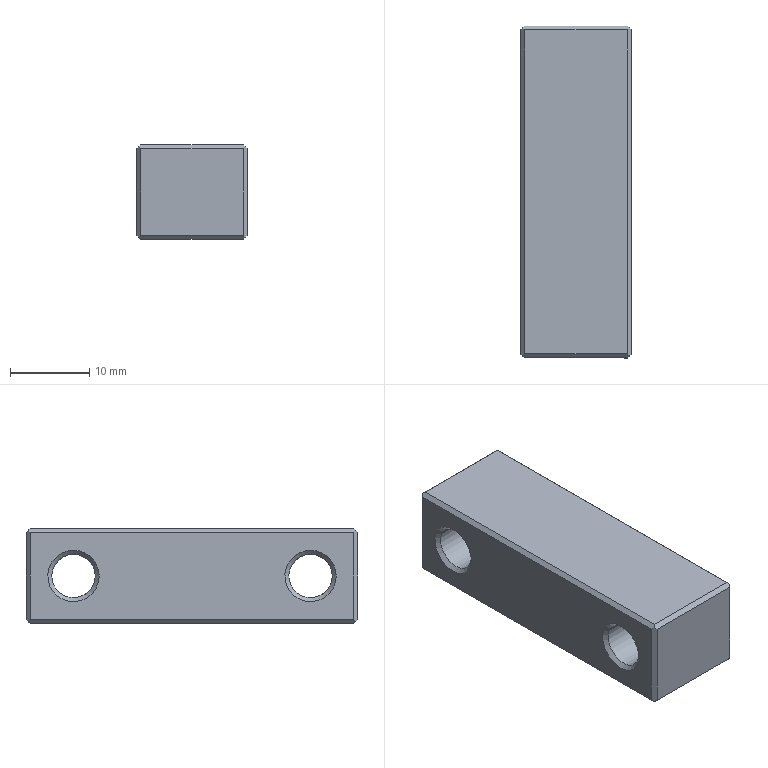Part | NX | 1 solid | 22 faces | box 14 x 42 x 12 mm | volume 6353 mm3 | plane 18 | cone 2 | cylinder 2 | commonest cylinder face diameters 5.5 x2
STEP:
#1=CARTESIAN_POINT('',(-39.202,6.721,154.477));
#2=VERTEX_POINT('',#1);
#3=CARTESIAN_POINT('',(-26.202,6.721,154.477));
#4=VERTEX_POINT('',#3);
#5=CARTESIAN_POINT('',(-1.702,6.721,154.477));
#6=DIRECTION('',(1.,0.,0.));
#7=VECTOR('',#6,1000.);
#8=LINE('',#5,#7);
#9=EDGE_CURVE('',#2,#4,#8,.T.);
#10=ORIENTED_EDGE('',*,*,#9,.T.);
#11=CARTESIAN_POINT('',(-26.202,47.721,154.477));
#12=VERTEX_POINT('',#11);
#13=CARTESIAN_POINT('',(-26.202,48.221,154.477));
#14=DIRECTION('',(0.,1.,0.));
#15=VECTOR('',#14,1000.);
#16=LINE('',#13,#15);
#17=EDGE_CURVE('',#4,#12,#16,.T.);
#18=ORIENTED_EDGE('',*,*,#17,.T.);
#19=CARTESIAN_POINT('',(-39.202,47.721,154.477));
#20=VERTEX_POINT('',#19);
#21=CARTESIAN_POINT('',(-1.702,47.721,154.477));
#22=DIRECTION('',(-1.,0.,0.));
#23=VECTOR('',#22,1000.);
#24=LINE('',#21,#23);
#25=EDGE_CURVE('',#12,#20,#24,.T.);
#26=ORIENTED_EDGE('',*,*,#25,.T.);
#27=CARTESIAN_POINT('',(-39.202,48.221,154.477));
#28=DIRECTION('',(0.,-1.,0.));
#29=VECTOR('',#28,1000.);
#30=LINE('',#27,#29);
#31=EDGE_CURVE('',#20,#2,#30,.T.);
#32=ORIENTED_EDGE('',*,*,#31,.T.);
#33=EDGE_LOOP('',(#10,#18,#26,#32));
#34=FACE_BOUND('',#33,.T.);
#35=CARTESIAN_POINT('',(-33.202,48.221,154.477));
#36=DIRECTION('',(0.,0.,-1.));
#37=DIRECTION('',(0.,-1.,0.));
#38=AXIS2_PLACEMENT_3D('',#35,#36,#37);
#39=PLANE('',#38);
#40=ADVANCED_FACE('',(#34),#39,.F.);
#41=CARTESIAN_POINT('',(-25.952,47.971,154.227));
#42=VERTEX_POINT('',#41);
#43=CARTESIAN_POINT('',(-41.43,32.492,169.705));
#44=DIRECTION('',(0.5774,0.5774,-0.5774));
#45=VECTOR('',#44,1000.);
#46=LINE('',#43,#45);
#47=EDGE_CURVE('',#12,#42,#46,.T.);
#48=ORIENTED_EDGE('',*,*,#47,.T.);
#49=CARTESIAN_POINT('',(-26.202,48.221,153.977));
#50=VERTEX_POINT('',#49);
#51=CARTESIAN_POINT('',(-29.702,51.721,150.477));
#52=DIRECTION('',(-0.5774,0.5774,-0.5774));
#53=VECTOR('',#52,1000.);
#54=LINE('',#51,#53);
#55=EDGE_CURVE('',#42,#50,#54,.T.);
#56=ORIENTED_EDGE('',*,*,#55,.T.);
#57=CARTESIAN_POINT('',(-39.202,48.221,153.977));
#58=VERTEX_POINT('',#57);
#59=CARTESIAN_POINT('',(-22.702,48.221,153.977));
#60=DIRECTION('',(1.,0.,0.));
#61=VECTOR('',#60,1000.);
#62=LINE('',#59,#61);
#63=EDGE_CURVE('',#58,#50,#62,.T.);
#64=ORIENTED_EDGE('',*,*,#63,.F.);
#65=CARTESIAN_POINT('',(-39.452,47.971,154.227));
#66=VERTEX_POINT('',#65);
#67=CARTESIAN_POINT('',(-39.202,48.221,153.977));
#68=DIRECTION('',(-0.5774,-0.5774,0.5774));
#69=VECTOR('',#68,1000.);
#70=LINE('',#67,#69);
#71=EDGE_CURVE('',#58,#66,#70,.T.);
#72=ORIENTED_EDGE('',*,*,#71,.T.);
#73=CARTESIAN_POINT('',(-39.452,47.971,154.227));
#74=DIRECTION('',(0.5774,-0.5774,0.5774));
#75=VECTOR('',#74,1000.);
#76=LINE('',#73,#75);
#77=EDGE_CURVE('',#66,#20,#76,.T.);
#78=ORIENTED_EDGE('',*,*,#77,.T.);
#79=ORIENTED_EDGE('',*,*,#25,.F.);
#80=EDGE_LOOP('',(#48,#56,#64,#72,#78,#79));
#81=FACE_BOUND('',#80,.T.);
#82=CARTESIAN_POINT('',(-1.702,48.221,153.977));
#83=DIRECTION('',(0.,-0.7071,-0.7071));
#84=DIRECTION('',(0.,-0.7071,0.7071));
#85=AXIS2_PLACEMENT_3D('',#82,#83,#84);
#86=PLANE('',#85);
#87=ADVANCED_FACE('',(#81),#86,.F.);
#88=CARTESIAN_POINT('',(-39.202,48.221,142.977));
#89=VERTEX_POINT('',#88);
#90=CARTESIAN_POINT('',(-39.202,48.221,142.477));
#91=DIRECTION('',(0.,0.,1.));
#92=VECTOR('',#91,1000.);
#93=LINE('',#90,#92);
#94=EDGE_CURVE('',#89,#58,#93,.T.);
#95=ORIENTED_EDGE('',*,*,#94,.F.);
#96=CARTESIAN_POINT('',(-39.452,47.971,142.727));
#97=VERTEX_POINT('',#96);
#98=CARTESIAN_POINT('',(-39.452,47.971,142.727));
#99=DIRECTION('',(0.5774,0.5774,0.5774));
#100=VECTOR('',#99,1000.);
#101=LINE('',#98,#100);
#102=EDGE_CURVE('',#97,#89,#101,.T.);
#103=ORIENTED_EDGE('',*,*,#102,.F.);
#104=CARTESIAN_POINT('',(-39.702,47.721,142.977));
#105=VERTEX_POINT('',#104);
#106=CARTESIAN_POINT('',(-39.702,47.721,142.977));
#107=DIRECTION('',(0.5774,0.5774,-0.5774));
#108=VECTOR('',#107,1000.);
#109=LINE('',#106,#108);
#110=EDGE_CURVE('',#105,#97,#109,.T.);
#111=ORIENTED_EDGE('',*,*,#110,.F.);
#112=CARTESIAN_POINT('',(-39.702,47.721,153.977));
#113=VERTEX_POINT('',#112);
#114=CARTESIAN_POINT('',(-39.702,47.721,142.977));
#115=DIRECTION('',(0.,0.,1.));
#116=VECTOR('',#115,1000.);
#117=LINE('',#114,#116);
#118=EDGE_CURVE('',#105,#113,#117,.T.);
#119=ORIENTED_EDGE('',*,*,#118,.T.);
#120=CARTESIAN_POINT('',(-39.702,47.721,153.977));
#121=DIRECTION('',(0.5774,0.5774,0.5774));
#122=VECTOR('',#121,1000.);
#123=LINE('',#120,#122);
#124=EDGE_CURVE('',#113,#66,#123,.T.);
#125=ORIENTED_EDGE('',*,*,#124,.T.);
#126=ORIENTED_EDGE('',*,*,#71,.F.);
#127=EDGE_LOOP('',(#95,#103,#111,#119,#125,#126));
#128=FACE_BOUND('',#127,.T.);
#129=CARTESIAN_POINT('',(-39.202,48.221,163.477));
#130=DIRECTION('',(0.7071,-0.7071,0.));
#131=DIRECTION('',(0.,0.,-1.));
#132=AXIS2_PLACEMENT_3D('',#129,#130,#131);
#133=PLANE('',#132);
#134=ADVANCED_FACE('',(#128),#133,.F.);
#135=ORIENTED_EDGE('',*,*,#31,.F.);
#136=ORIENTED_EDGE('',*,*,#77,.F.);
#137=ORIENTED_EDGE('',*,*,#124,.F.);
#138=CARTESIAN_POINT('',(-39.702,6.721,153.977));
#139=VERTEX_POINT('',#138);
#140=CARTESIAN_POINT('',(-39.702,48.221,153.977));
#141=DIRECTION('',(0.,-1.,0.));
#142=VECTOR('',#141,1000.);
#143=LINE('',#140,#142);
#144=EDGE_CURVE('',#113,#139,#143,.T.);
#145=ORIENTED_EDGE('',*,*,#144,.T.);
#146=CARTESIAN_POINT('',(-39.452,6.471,154.227));
#147=VERTEX_POINT('',#146);
#148=CARTESIAN_POINT('',(-39.702,6.721,153.977));
#149=DIRECTION('',(0.5774,-0.5774,0.5774));
#150=VECTOR('',#149,1000.);
#151=LINE('',#148,#150);
#152=EDGE_CURVE('',#139,#147,#151,.T.);
#153=ORIENTED_EDGE('',*,*,#152,.T.);
#154=CARTESIAN_POINT('',(-39.452,6.471,154.227));
#155=DIRECTION('',(0.5774,0.5774,0.5774));
#156=VECTOR('',#155,1000.);
#157=LINE('',#154,#156);
#158=EDGE_CURVE('',#147,#2,#157,.T.);
#159=ORIENTED_EDGE('',*,*,#158,.T.);
#160=EDGE_LOOP('',(#135,#136,#137,#145,#153,#159));
#161=FACE_BOUND('',#160,.T.);
#162=CARTESIAN_POINT('',(-39.702,48.221,153.977));
#163=DIRECTION('',(0.7071,0.,-0.7071));
#164=DIRECTION('',(0.,-1.,0.));
#165=AXIS2_PLACEMENT_3D('',#162,#163,#164);
#166=PLANE('',#165);
#167=ADVANCED_FACE('',(#161),#166,.F.);
#168=CARTESIAN_POINT('',(-39.202,6.221,142.977));
#169=VERTEX_POINT('',#168);
#170=CARTESIAN_POINT('',(-39.202,6.221,153.977));
#171=VERTEX_POINT('',#170);
#172=CARTESIAN_POINT('',(-39.202,6.221,142.477));
#173=DIRECTION('',(0.,0.,1.));
#174=VECTOR('',#173,1000.);
#175=LINE('',#172,#174);
#176=EDGE_CURVE('',#169,#171,#175,.T.);
#177=ORIENTED_EDGE('',*,*,#176,.T.);
#178=CARTESIAN_POINT('',(-39.202,6.221,153.977));
#179=DIRECTION('',(-0.5774,0.5774,0.5774));
#180=VECTOR('',#179,1000.);
#181=LINE('',#178,#180);
#182=EDGE_CURVE('',#171,#147,#181,.T.);
#183=ORIENTED_EDGE('',*,*,#182,.T.);
#184=ORIENTED_EDGE('',*,*,#152,.F.);
#185=CARTESIAN_POINT('',(-39.702,6.721,142.977));
#186=VERTEX_POINT('',#185);
#187=CARTESIAN_POINT('',(-39.702,6.721,142.977));
#188=DIRECTION('',(0.,0.,-1.));
#189=VECTOR('',#188,1000.);
#190=LINE('',#187,#189);
#191=EDGE_CURVE('',#139,#186,#190,.T.);
#192=ORIENTED_EDGE('',*,*,#191,.T.);
#193=CARTESIAN_POINT('',(-39.452,6.471,142.727));
#194=VERTEX_POINT('',#193);
#195=CARTESIAN_POINT('',(-39.452,6.471,142.727));
#196=DIRECTION('',(-0.5774,0.5774,0.5774));
#197=VECTOR('',#196,1000.);
#198=LINE('',#195,#197);
#199=EDGE_CURVE('',#194,#186,#198,.T.);
#200=ORIENTED_EDGE('',*,*,#199,.F.);
#201=CARTESIAN_POINT('',(-39.202,6.221,142.977));
#202=DIRECTION('',(-0.5774,0.5774,-0.5774));
#203=VECTOR('',#202,1000.);
#204=LINE('',#201,#203);
#205=EDGE_CURVE('',#169,#194,#204,.T.);
#206=ORIENTED_EDGE('',*,*,#205,.F.);
#207=EDGE_LOOP('',(#177,#183,#184,#192,#200,#206));
#208=FACE_BOUND('',#207,.T.);
#209=CARTESIAN_POINT('',(-39.702,6.721,163.477));
#210=DIRECTION('',(0.7071,0.7071,0.));
#211=DIRECTION('',(0.,0.,-1.));
#212=AXIS2_PLACEMENT_3D('',#209,#210,#211);
#213=PLANE('',#212);
#214=ADVANCED_FACE('',(#208),#213,.F.);
#215=CARTESIAN_POINT('',(-26.202,6.221,153.977));
#216=VERTEX_POINT('',#215);
#217=CARTESIAN_POINT('',(-22.702,6.221,153.977));
#218=DIRECTION('',(1.,0.,0.));
#219=VECTOR('',#218,1000.);
#220=LINE('',#217,#219);
#221=EDGE_CURVE('',#171,#216,#220,.T.);
#222=ORIENTED_EDGE('',*,*,#221,.T.);
#223=CARTESIAN_POINT('',(-25.952,6.471,154.227));
#224=VERTEX_POINT('',#223);
#225=CARTESIAN_POINT('',(-30.035,2.387,150.144));
#226=DIRECTION('',(0.5774,0.5774,0.5774));
#227=VECTOR('',#226,1000.);
#228=LINE('',#225,#227);
#229=EDGE_CURVE('',#216,#224,#228,.T.);
#230=ORIENTED_EDGE('',*,*,#229,.T.);
#231=CARTESIAN_POINT('',(-23.974,4.492,152.249));
#232=DIRECTION('',(-0.5774,0.5774,0.5774));
#233=VECTOR('',#232,1000.);
#234=LINE('',#231,#233);
#235=EDGE_CURVE('',#224,#4,#234,.T.);
#236=ORIENTED_EDGE('',*,*,#235,.T.);
#237=ORIENTED_EDGE('',*,*,#9,.F.);
#238=ORIENTED_EDGE('',*,*,#158,.F.);
#239=ORIENTED_EDGE('',*,*,#182,.F.);
#240=EDGE_LOOP('',(#222,#230,#236,#237,#238,#239));
#241=FACE_BOUND('',#240,.T.);
#242=CARTESIAN_POINT('',(-1.702,6.721,154.477));
#243=DIRECTION('',(0.,0.7071,-0.7071));
#244=DIRECTION('',(-1.,0.,0.));
#245=AXIS2_PLACEMENT_3D('',#242,#243,#244);
#246=PLANE('',#245);
#247=ADVANCED_FACE('',(#241),#246,.F.);
#248=ORIENTED_EDGE('',*,*,#63,.T.);
#249=CARTESIAN_POINT('',(-26.202,48.221,142.977));
#250=VERTEX_POINT('',#249);
#251=CARTESIAN_POINT('',(-26.202,48.221,142.977));
#252=DIRECTION('',(0.,0.,-1.));
#253=VECTOR('',#252,1000.);
#254=LINE('',#251,#253);
#255=EDGE_CURVE('',#50,#250,#254,.T.);
#256=ORIENTED_EDGE('',*,*,#255,.T.);
#257=CARTESIAN_POINT('',(-1.702,48.221,142.977));
#258=DIRECTION('',(-1.,0.,0.));
#259=VECTOR('',#258,1000.);
#260=LINE('',#257,#259);
#261=EDGE_CURVE('',#250,#89,#260,.T.);
#262=ORIENTED_EDGE('',*,*,#261,.T.);
#263=ORIENTED_EDGE('',*,*,#94,.T.);
#264=EDGE_LOOP('',(#248,#256,#262,#263));
#265=FACE_BOUND('',#264,.T.);
#266=CARTESIAN_POINT('',(-22.702,48.221,142.477));
#267=DIRECTION('',(0.,1.,0.));
#268=DIRECTION('',(1.,0.,0.));
#269=AXIS2_PLACEMENT_3D('',#266,#267,#268);
#270=PLANE('',#269);
#271=ADVANCED_FACE('',(#265),#270,.T.);
#272=CARTESIAN_POINT('',(-39.702,42.221,151.727));
#273=VERTEX_POINT('',#272);
#274=CARTESIAN_POINT('',(-39.702,42.221,148.477));
#275=DIRECTION('',(-1.,0.,0.));
#276=DIRECTION('',(0.,0.,1.));
#277=AXIS2_PLACEMENT_3D('',#274,#275,#276);
#278=CIRCLE('',#277,3.25);
#279=EDGE_CURVE('',#273,#273,#278,.T.);
#280=ORIENTED_EDGE('',*,*,#279,.F.);
#281=EDGE_LOOP('',(#280));
#282=FACE_BOUND('',#281,.T.);
#283=CARTESIAN_POINT('',(-39.702,12.221,151.727));
#284=VERTEX_POINT('',#283);
#285=CARTESIAN_POINT('',(-39.702,12.221,148.477));
#286=DIRECTION('',(-1.,0.,0.));
#287=DIRECTION('',(0.,0.,1.));
#288=AXIS2_PLACEMENT_3D('',#285,#286,#287);
#289=CIRCLE('',#288,3.25);
#290=EDGE_CURVE('',#284,#284,#289,.T.);
#291=ORIENTED_EDGE('',*,*,#290,.F.);
#292=EDGE_LOOP('',(#291));
#293=FACE_BOUND('',#292,.T.);
#294=ORIENTED_EDGE('',*,*,#144,.F.);
#295=ORIENTED_EDGE('',*,*,#118,.F.);
#296=CARTESIAN_POINT('',(-39.702,48.221,142.977));
#297=DIRECTION('',(0.,-1.,0.));
#298=VECTOR('',#297,1000.);
#299=LINE('',#296,#298);
#300=EDGE_CURVE('',#105,#186,#299,.T.);
#301=ORIENTED_EDGE('',*,*,#300,.T.);
#302=ORIENTED_EDGE('',*,*,#191,.F.);
#303=EDGE_LOOP('',(#294,#295,#301,#302));
#304=FACE_BOUND('',#303,.T.);
#305=CARTESIAN_POINT('',(-39.702,48.221,142.977));
#306=DIRECTION('',(1.,0.,0.));
#307=DIRECTION('',(0.,0.,1.));
#308=AXIS2_PLACEMENT_3D('',#305,#306,#307);
#309=PLANE('',#308);
#310=ADVANCED_FACE('',(#282,#293,#304),#309,.F.);
#311=CARTESIAN_POINT('',(-26.202,6.221,142.977));
#312=VERTEX_POINT('',#311);
#313=CARTESIAN_POINT('',(-1.702,6.221,142.977));
#314=DIRECTION('',(1.,0.,0.));
#315=VECTOR('',#314,1000.);
#316=LINE('',#313,#315);
#317=EDGE_CURVE('',#169,#312,#316,.T.);
#318=ORIENTED_EDGE('',*,*,#317,.T.);
#319=CARTESIAN_POINT('',(-26.202,6.221,142.477));
#320=DIRECTION('',(0.,0.,1.));
#321=VECTOR('',#320,1000.);
#322=LINE('',#319,#321);
#323=EDGE_CURVE('',#312,#216,#322,.T.);
#324=ORIENTED_EDGE('',*,*,#323,.T.);
#325=ORIENTED_EDGE('',*,*,#221,.F.);
#326=ORIENTED_EDGE('',*,*,#176,.F.);
#327=EDGE_LOOP('',(#318,#324,#325,#326));
#328=FACE_BOUND('',#327,.T.);
#329=CARTESIAN_POINT('',(-22.702,6.221,142.477));
#330=DIRECTION('',(0.,1.,0.));
#331=DIRECTION('',(1.,0.,0.));
#332=AXIS2_PLACEMENT_3D('',#329,#330,#331);
#333=PLANE('',#332);
#334=ADVANCED_FACE('',(#328),#333,.F.);
#335=ORIENTED_EDGE('',*,*,#261,.F.);
#336=CARTESIAN_POINT('',(-25.952,47.971,142.727));
#337=VERTEX_POINT('',#336);
#338=CARTESIAN_POINT('',(-25.702,47.721,142.477));
#339=DIRECTION('',(0.5774,-0.5774,-0.5774));
#340=VECTOR('',#339,1000.);
#341=LINE('',#338,#340);
#342=EDGE_CURVE('',#250,#337,#341,.T.);
#343=ORIENTED_EDGE('',*,*,#342,.T.);
#344=CARTESIAN_POINT('',(-26.202,47.721,142.477));
#345=VERTEX_POINT('',#344);
#346=CARTESIAN_POINT('',(-26.035,47.887,142.644));
#347=DIRECTION('',(-0.5774,-0.5774,-0.5774));
#348=VECTOR('',#347,1000.);
#349=LINE('',#346,#348);
#350=EDGE_CURVE('',#337,#345,#349,.T.);
#351=ORIENTED_EDGE('',*,*,#350,.T.);
#352=CARTESIAN_POINT('',(-39.202,47.721,142.477));
#353=VERTEX_POINT('',#352);
#354=CARTESIAN_POINT('',(-12.202,47.721,142.477));
#355=DIRECTION('',(-1.,0.,0.));
#356=VECTOR('',#355,1000.);
#357=LINE('',#354,#356);
#358=EDGE_CURVE('',#345,#353,#357,.T.);
#359=ORIENTED_EDGE('',*,*,#358,.T.);
#360=CARTESIAN_POINT('',(-39.202,47.721,142.477));
#361=DIRECTION('',(-0.5774,0.5774,0.5774));
#362=VECTOR('',#361,1000.);
#363=LINE('',#360,#362);
#364=EDGE_CURVE('',#353,#97,#363,.T.);
#365=ORIENTED_EDGE('',*,*,#364,.T.);
#366=ORIENTED_EDGE('',*,*,#102,.T.);
#367=EDGE_LOOP('',(#335,#343,#351,#359,#365,#366));
#368=FACE_BOUND('',#367,.T.);
#369=CARTESIAN_POINT('',(-1.702,47.721,142.477));
#370=DIRECTION('',(0.,-0.7071,0.7071));
#371=DIRECTION('',(-1.,0.,0.));
#372=AXIS2_PLACEMENT_3D('',#369,#370,#371);
#373=PLANE('',#372);
#374=ADVANCED_FACE('',(#368),#373,.F.);
#375=ORIENTED_EDGE('',*,*,#199,.T.);
#376=ORIENTED_EDGE('',*,*,#300,.F.);
#377=ORIENTED_EDGE('',*,*,#110,.T.);
#378=ORIENTED_EDGE('',*,*,#364,.F.);
#379=CARTESIAN_POINT('',(-39.202,6.721,142.477));
#380=VERTEX_POINT('',#379);
#381=CARTESIAN_POINT('',(-39.202,48.221,142.477));
#382=DIRECTION('',(0.,-1.,0.));
#383=VECTOR('',#382,1000.);
#384=LINE('',#381,#383);
#385=EDGE_CURVE('',#353,#380,#384,.T.);
#386=ORIENTED_EDGE('',*,*,#385,.T.);
#387=CARTESIAN_POINT('',(-39.202,6.721,142.477));
#388=DIRECTION('',(-0.5774,-0.5774,0.5774));
#389=VECTOR('',#388,1000.);
#390=LINE('',#387,#389);
#391=EDGE_CURVE('',#380,#194,#390,.T.);
#392=ORIENTED_EDGE('',*,*,#391,.T.);
#393=EDGE_LOOP('',(#375,#376,#377,#378,#386,#392));
#394=FACE_BOUND('',#393,.T.);
#395=CARTESIAN_POINT('',(-39.202,48.221,142.477));
#396=DIRECTION('',(0.7071,0.,0.7071));
#397=DIRECTION('',(0.,-1.,0.));
#398=AXIS2_PLACEMENT_3D('',#395,#396,#397);
#399=PLANE('',#398);
#400=ADVANCED_FACE('',(#394),#399,.F.);
#401=CARTESIAN_POINT('',(-26.202,6.721,142.477));
#402=VERTEX_POINT('',#401);
#403=CARTESIAN_POINT('',(-12.202,6.721,142.477));
#404=DIRECTION('',(1.,0.,0.));
#405=VECTOR('',#404,1000.);
#406=LINE('',#403,#405);
#407=EDGE_CURVE('',#380,#402,#406,.T.);
#408=ORIENTED_EDGE('',*,*,#407,.T.);
#409=CARTESIAN_POINT('',(-25.952,6.471,142.727));
#410=VERTEX_POINT('',#409);
#411=CARTESIAN_POINT('',(-40.035,20.554,128.644));
#412=DIRECTION('',(0.5774,-0.5774,0.5774));
#413=VECTOR('',#412,1000.);
#414=LINE('',#411,#413);
#415=EDGE_CURVE('',#402,#410,#414,.T.);
#416=ORIENTED_EDGE('',*,*,#415,.T.);
#417=CARTESIAN_POINT('',(-26.035,6.387,142.81));
#418=DIRECTION('',(-0.5774,-0.5774,0.5774));
#419=VECTOR('',#418,1000.);
#420=LINE('',#417,#419);
#421=EDGE_CURVE('',#410,#312,#420,.T.);
#422=ORIENTED_EDGE('',*,*,#421,.T.);
#423=ORIENTED_EDGE('',*,*,#317,.F.);
#424=ORIENTED_EDGE('',*,*,#205,.T.);
#425=ORIENTED_EDGE('',*,*,#391,.F.);
#426=EDGE_LOOP('',(#408,#416,#422,#423,#424,#425));
#427=FACE_BOUND('',#426,.T.);
#428=CARTESIAN_POINT('',(-1.702,6.221,142.977));
#429=DIRECTION('',(0.,0.7071,0.7071));
#430=DIRECTION('',(1.,0.,0.));
#431=AXIS2_PLACEMENT_3D('',#428,#429,#430);
#432=PLANE('',#431);
#433=ADVANCED_FACE('',(#427),#432,.F.);
#434=ORIENTED_EDGE('',*,*,#358,.F.);
#435=CARTESIAN_POINT('',(-26.202,48.221,142.477));
#436=DIRECTION('',(0.,-1.,0.));
#437=VECTOR('',#436,1000.);
#438=LINE('',#435,#437);
#439=EDGE_CURVE('',#345,#402,#438,.T.);
#440=ORIENTED_EDGE('',*,*,#439,.T.);
#441=ORIENTED_EDGE('',*,*,#407,.F.);
#442=ORIENTED_EDGE('',*,*,#385,.F.);
#443=EDGE_LOOP('',(#434,#440,#441,#442));
#444=FACE_BOUND('',#443,.T.);
#445=CARTESIAN_POINT('',(-12.202,48.221,142.477));
#446=DIRECTION('',(0.,0.,1.));
#447=DIRECTION('',(1.,0.,0.));
#448=AXIS2_PLACEMENT_3D('',#445,#446,#447);
#449=PLANE('',#448);
#450=ADVANCED_FACE('',(#444),#449,.F.);
#451=CARTESIAN_POINT('',(-25.702,6.721,142.977));
#452=VERTEX_POINT('',#451);
#453=CARTESIAN_POINT('',(-25.702,47.721,142.977));
#454=VERTEX_POINT('',#453);
#455=CARTESIAN_POINT('',(-25.702,1.036,142.977));
#456=DIRECTION('',(0.,1.,0.));
#457=VECTOR('',#456,1000.);
#458=LINE('',#455,#457);
#459=EDGE_CURVE('',#452,#454,#458,.T.);
#460=ORIENTED_EDGE('',*,*,#459,.T.);
#461=CARTESIAN_POINT('',(-25.702,47.721,153.977));
#462=VERTEX_POINT('',#461);
#463=CARTESIAN_POINT('',(-25.702,47.721,153.977));
#464=DIRECTION('',(0.,0.,1.));
#465=VECTOR('',#464,1000.);
#466=LINE('',#463,#465);
#467=EDGE_CURVE('',#454,#462,#466,.T.);
#468=ORIENTED_EDGE('',*,*,#467,.T.);
#469=CARTESIAN_POINT('',(-25.702,6.721,153.977));
#470=VERTEX_POINT('',#469);
#471=CARTESIAN_POINT('',(-25.702,1.036,153.977));
#472=DIRECTION('',(0.,-1.,0.));
#473=VECTOR('',#472,1000.);
#474=LINE('',#471,#473);
#475=EDGE_CURVE('',#462,#470,#474,.T.);
#476=ORIENTED_EDGE('',*,*,#475,.T.);
#477=CARTESIAN_POINT('',(-25.702,6.721,142.477));
#478=DIRECTION('',(0.,0.,-1.));
#479=VECTOR('',#478,1000.);
#480=LINE('',#477,#479);
#481=EDGE_CURVE('',#470,#452,#480,.T.);
#482=ORIENTED_EDGE('',*,*,#481,.T.);
#483=EDGE_LOOP('',(#460,#468,#476,#482));
#484=FACE_BOUND('',#483,.T.);
#485=CARTESIAN_POINT('',(-25.702,42.221,151.227));
#486=VERTEX_POINT('',#485);
#487=CARTESIAN_POINT('',(-25.702,42.221,148.477));
#488=DIRECTION('',(1.,0.,0.));
#489=DIRECTION('',(0.,0.,1.));
#490=AXIS2_PLACEMENT_3D('',#487,#488,#489);
#491=CIRCLE('',#490,2.75);
#492=EDGE_CURVE('',#486,#486,#491,.T.);
#493=ORIENTED_EDGE('',*,*,#492,.F.);
#494=EDGE_LOOP('',(#493));
#495=FACE_BOUND('',#494,.T.);
#496=CARTESIAN_POINT('',(-25.702,12.221,151.227));
#497=VERTEX_POINT('',#496);
#498=CARTESIAN_POINT('',(-25.702,12.221,148.477));
#499=DIRECTION('',(1.,0.,0.));
#500=DIRECTION('',(0.,0.,1.));
#501=AXIS2_PLACEMENT_3D('',#498,#499,#500);
#502=CIRCLE('',#501,2.75);
#503=EDGE_CURVE('',#497,#497,#502,.T.);
#504=ORIENTED_EDGE('',*,*,#503,.F.);
#505=EDGE_LOOP('',(#504));
#506=FACE_BOUND('',#505,.T.);
#507=CARTESIAN_POINT('',(-25.702,1.036,142.477));
#508=DIRECTION('',(-1.,0.,0.));
#509=DIRECTION('',(0.,0.,1.));
#510=AXIS2_PLACEMENT_3D('',#507,#508,#509);
#511=PLANE('',#510);
#512=ADVANCED_FACE('',(#484,#495,#506),#511,.F.);
#513=ORIENTED_EDGE('',*,*,#323,.F.);
#514=ORIENTED_EDGE('',*,*,#421,.F.);
#515=CARTESIAN_POINT('',(-12.202,20.221,156.477));
#516=DIRECTION('',(-0.5774,-0.5774,-0.5774));
#517=VECTOR('',#516,1000.);
#518=LINE('',#515,#517);
#519=EDGE_CURVE('',#452,#410,#518,.T.);
#520=ORIENTED_EDGE('',*,*,#519,.F.);
#521=ORIENTED_EDGE('',*,*,#481,.F.);
#522=CARTESIAN_POINT('',(-22.202,10.221,150.477));
#523=DIRECTION('',(0.5774,0.5774,-0.5774));
#524=VECTOR('',#523,1000.);
#525=LINE('',#522,#524);
#526=EDGE_CURVE('',#224,#470,#525,.T.);
#527=ORIENTED_EDGE('',*,*,#526,.F.);
#528=ORIENTED_EDGE('',*,*,#229,.F.);
#529=EDGE_LOOP('',(#513,#514,#520,#521,#527,#528));
#530=FACE_BOUND('',#529,.T.);
#531=CARTESIAN_POINT('',(-26.202,6.221,142.477));
#532=DIRECTION('',(-0.7071,0.7071,0.));
#533=DIRECTION('',(0.,0.,1.));
#534=AXIS2_PLACEMENT_3D('',#531,#532,#533);
#535=PLANE('',#534);
#536=ADVANCED_FACE('',(#530),#535,.F.);
#537=ORIENTED_EDGE('',*,*,#439,.F.);
#538=ORIENTED_EDGE('',*,*,#350,.F.);
#539=CARTESIAN_POINT('',(-25.869,47.887,142.81));
#540=DIRECTION('',(-0.5774,0.5774,-0.5774));
#541=VECTOR('',#540,1000.);
#542=LINE('',#539,#541);
#543=EDGE_CURVE('',#454,#337,#542,.T.);
#544=ORIENTED_EDGE('',*,*,#543,.F.);
#545=ORIENTED_EDGE('',*,*,#459,.F.);
#546=ORIENTED_EDGE('',*,*,#519,.T.);
#547=ORIENTED_EDGE('',*,*,#415,.F.);
#548=EDGE_LOOP('',(#537,#538,#544,#545,#546,#547));
#549=FACE_BOUND('',#548,.T.);
#550=CARTESIAN_POINT('',(-26.202,48.221,142.477));
#551=DIRECTION('',(-0.7071,0.,0.7071));
#552=DIRECTION('',(0.,1.,0.));
#553=AXIS2_PLACEMENT_3D('',#550,#551,#552);
#554=PLANE('',#553);
#555=ADVANCED_FACE('',(#549),#554,.F.);
#556=ORIENTED_EDGE('',*,*,#526,.T.);
#557=ORIENTED_EDGE('',*,*,#475,.F.);
#558=CARTESIAN_POINT('',(-10.14,32.159,138.415));
#559=DIRECTION('',(0.5774,-0.5774,-0.5774));
#560=VECTOR('',#559,1000.);
#561=LINE('',#558,#560);
#562=EDGE_CURVE('',#42,#462,#561,.T.);
#563=ORIENTED_EDGE('',*,*,#562,.F.);
#564=ORIENTED_EDGE('',*,*,#47,.F.);
#565=ORIENTED_EDGE('',*,*,#17,.F.);
#566=ORIENTED_EDGE('',*,*,#235,.F.);
#567=EDGE_LOOP('',(#556,#557,#563,#564,#565,#566));
#568=FACE_BOUND('',#567,.T.);
#569=CARTESIAN_POINT('',(-25.702,1.036,153.977));
#570=DIRECTION('',(-0.7071,0.,-0.7071));
#571=DIRECTION('',(-0.7071,0.,0.7071));
#572=AXIS2_PLACEMENT_3D('',#569,#570,#571);
#573=PLANE('',#572);
#574=ADVANCED_FACE('',(#568),#573,.F.);
#575=ORIENTED_EDGE('',*,*,#342,.F.);
#576=ORIENTED_EDGE('',*,*,#255,.F.);
#577=ORIENTED_EDGE('',*,*,#55,.F.);
#578=ORIENTED_EDGE('',*,*,#562,.T.);
#579=ORIENTED_EDGE('',*,*,#467,.F.);
#580=ORIENTED_EDGE('',*,*,#543,.T.);
#581=EDGE_LOOP('',(#575,#576,#577,#578,#579,#580));
#582=FACE_BOUND('',#581,.T.);
#583=CARTESIAN_POINT('',(-25.702,47.721,142.477));
#584=DIRECTION('',(0.7071,0.7071,0.));
#585=DIRECTION('',(0.,0.,-1.));
#586=AXIS2_PLACEMENT_3D('',#583,#584,#585);
#587=PLANE('',#586);
#588=ADVANCED_FACE('',(#582),#587,.T.);
#589=ORIENTED_EDGE('',*,*,#279,.T.);
#590=EDGE_LOOP('',(#589));
#591=FACE_BOUND('',#590,.T.);
#592=CARTESIAN_POINT('',(-39.202,39.471,148.477));
#593=VERTEX_POINT('',#592);
#594=CARTESIAN_POINT('',(-39.202,42.221,148.477));
#595=DIRECTION('',(-1.,0.,0.));
#596=DIRECTION('',(0.,-1.,0.));
#597=AXIS2_PLACEMENT_3D('',#594,#595,#596);
#598=CIRCLE('',#597,2.75);
#599=EDGE_CURVE('',#593,#593,#598,.T.);
#600=ORIENTED_EDGE('',*,*,#599,.F.);
#601=EDGE_LOOP('',(#600));
#602=FACE_BOUND('',#601,.T.);
#603=CARTESIAN_POINT('',(-39.702,42.221,148.477));
#604=DIRECTION('',(-1.,0.,0.));
#605=DIRECTION('',(0.,0.,-1.));
#606=AXIS2_PLACEMENT_3D('',#603,#604,#605);
#607=CONICAL_SURFACE('',#606,3.25,0.7854);
#608=ADVANCED_FACE('',(#591,#602),#607,.F.);
#609=ORIENTED_EDGE('',*,*,#290,.T.);
#610=EDGE_LOOP('',(#609));
#611=FACE_BOUND('',#610,.T.);
#612=CARTESIAN_POINT('',(-39.202,9.471,148.477));
#613=VERTEX_POINT('',#612);
#614=CARTESIAN_POINT('',(-39.202,12.221,148.477));
#615=DIRECTION('',(-1.,0.,0.));
#616=DIRECTION('',(0.,-1.,0.));
#617=AXIS2_PLACEMENT_3D('',#614,#615,#616);
#618=CIRCLE('',#617,2.75);
#619=EDGE_CURVE('',#613,#613,#618,.T.);
#620=ORIENTED_EDGE('',*,*,#619,.F.);
#621=EDGE_LOOP('',(#620));
#622=FACE_BOUND('',#621,.T.);
#623=CARTESIAN_POINT('',(-39.702,12.221,148.477));
#624=DIRECTION('',(-1.,0.,0.));
#625=DIRECTION('',(0.,0.,-1.));
#626=AXIS2_PLACEMENT_3D('',#623,#624,#625);
#627=CONICAL_SURFACE('',#626,3.25,0.7854);
#628=ADVANCED_FACE('',(#611,#622),#627,.F.);
#629=ORIENTED_EDGE('',*,*,#599,.T.);
#630=EDGE_LOOP('',(#629));
#631=FACE_BOUND('',#630,.T.);
#632=ORIENTED_EDGE('',*,*,#492,.T.);
#633=EDGE_LOOP('',(#632));
#634=FACE_BOUND('',#633,.T.);
#635=CARTESIAN_POINT('',(-33.702,42.221,148.477));
#636=DIRECTION('',(1.,0.,0.));
#637=DIRECTION('',(0.,0.,1.));
#638=AXIS2_PLACEMENT_3D('',#635,#636,#637);
#639=CYLINDRICAL_SURFACE('',#638,2.75);
#640=ADVANCED_FACE('',(#631,#634),#639,.F.);
#641=ORIENTED_EDGE('',*,*,#619,.T.);
#642=EDGE_LOOP('',(#641));
#643=FACE_BOUND('',#642,.T.);
#644=ORIENTED_EDGE('',*,*,#503,.T.);
#645=EDGE_LOOP('',(#644));
#646=FACE_BOUND('',#645,.T.);
#647=CARTESIAN_POINT('',(-33.702,12.221,148.477));
#648=DIRECTION('',(1.,0.,0.));
#649=DIRECTION('',(0.,0.,1.));
#650=AXIS2_PLACEMENT_3D('',#647,#648,#649);
#651=CYLINDRICAL_SURFACE('',#650,2.75);
#652=ADVANCED_FACE('',(#643,#646),#651,.F.);
#653=CLOSED_SHELL('',(#40,#87,#134,#167,#214,#247,#271,#310,#334,#374,#400,#433,#450,#512,#536,#555,#574,#588,#608,#628,#640,#652));
#654=MANIFOLD_SOLID_BREP('',#653);
#655=(LENGTH_UNIT()NAMED_UNIT(*)SI_UNIT(.MILLI.,.METRE.));
#656=UNCERTAINTY_MEASURE_WITH_UNIT(LENGTH_MEASURE(0.00001),#655,'','');
#657=(NAMED_UNIT(*)PLANE_ANGLE_UNIT()SI_UNIT($,.RADIAN.));
#658=(NAMED_UNIT(*)SI_UNIT($,.STERADIAN.)SOLID_ANGLE_UNIT());
#659=(GEOMETRIC_REPRESENTATION_CONTEXT(3)GLOBAL_UNCERTAINTY_ASSIGNED_CONTEXT((#656))GLOBAL_UNIT_ASSIGNED_CONTEXT((#655,#657,#658))REPRESENTATION_CONTEXT('',''));
#660=ADVANCED_BREP_SHAPE_REPRESENTATION('',(#654),#659);